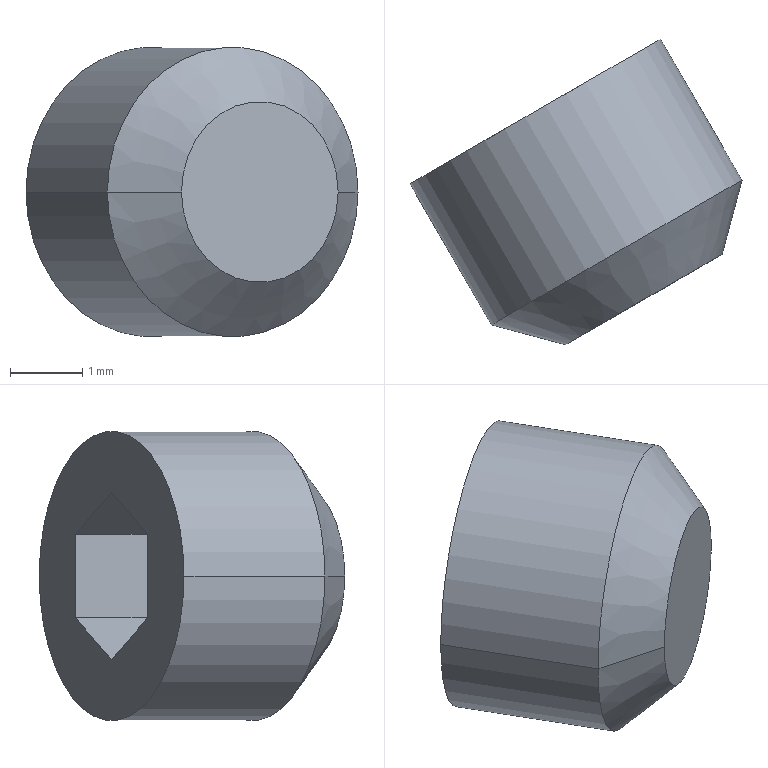Part | SolidWorks | features BaseBody 1 | 1 solid | 20 faces | box 4.589 x 4.223 x 4 mm | volume 28.806 mm3 | plane 14 | cone 4 | cylinder 2 | commonest cylinder face diameters 4 x2
STEP:
#1=CARTESIAN_POINT('',(315.686,1754.162,-1178.57));
#2=VERTEX_POINT('',#1);
#3=CARTESIAN_POINT('',(319.15,1756.162,-1178.57));
#4=VERTEX_POINT('',#3);
#5=CARTESIAN_POINT('',(317.418,1755.162,-1178.57));
#6=DIRECTION('',(-0.5,0.866,0.));
#7=DIRECTION('',(-0.866,-0.5,0.));
#8=AXIS2_PLACEMENT_3D('',#5,#6,#7);
#9=CIRCLE('',#8,2.);
#10=EDGE_CURVE('',#2,#4,#9,.T.);
#11=ORIENTED_EDGE('',*,*,#10,.T.);
#12=CARTESIAN_POINT('',(318.025,1758.11,-1178.57));
#13=VERTEX_POINT('',#12);
#14=CARTESIAN_POINT('',(318.025,1758.11,-1178.57));
#15=DIRECTION('',(-0.5,0.866,0.));
#16=VECTOR('',#15,1000.);
#17=LINE('',#14,#16);
#18=EDGE_CURVE('',#4,#13,#17,.T.);
#19=ORIENTED_EDGE('',*,*,#18,.T.);
#20=CARTESIAN_POINT('',(314.561,1756.11,-1178.57));
#21=VERTEX_POINT('',#20);
#22=CARTESIAN_POINT('',(316.293,1757.11,-1178.57));
#23=DIRECTION('',(0.5,-0.866,0.));
#24=DIRECTION('',(-0.866,-0.5,0.));
#25=AXIS2_PLACEMENT_3D('',#22,#23,#24);
#26=CIRCLE('',#25,2.);
#27=EDGE_CURVE('',#13,#21,#26,.T.);
#28=ORIENTED_EDGE('',*,*,#27,.T.);
#29=CARTESIAN_POINT('',(314.561,1756.11,-1178.57));
#30=DIRECTION('',(-0.5,0.866,0.));
#31=VECTOR('',#30,1000.);
#32=LINE('',#29,#31);
#33=EDGE_CURVE('',#2,#21,#32,.T.);
#34=ORIENTED_EDGE('',*,*,#33,.F.);
#35=EDGE_LOOP('',(#11,#19,#28,#34));
#36=FACE_OUTER_BOUND('',#35,.T.);
#37=CARTESIAN_POINT('',(316.293,1757.11,-1178.57));
#38=DIRECTION('',(-0.5,0.866,0.));
#39=DIRECTION('',(-0.866,-0.5,0.));
#40=AXIS2_PLACEMENT_3D('',#37,#38,#39);
#41=CYLINDRICAL_SURFACE('',#40,2.);
#42=ADVANCED_FACE('',(#36),#41,.T.);
#43=CARTESIAN_POINT('',(316.71,1753.887,-1178.57));
#44=VERTEX_POINT('',#43);
#45=CARTESIAN_POINT('',(318.875,1755.137,-1178.57));
#46=VERTEX_POINT('',#45);
#47=CARTESIAN_POINT('',(317.793,1754.512,-1178.57));
#48=DIRECTION('',(-0.5,0.866,0.));
#49=DIRECTION('',(-0.866,-0.5,0.));
#50=AXIS2_PLACEMENT_3D('',#47,#48,#49);
#51=CIRCLE('',#50,1.25);
#52=EDGE_CURVE('',#44,#46,#51,.T.);
#53=ORIENTED_EDGE('',*,*,#52,.T.);
#54=CARTESIAN_POINT('',(319.15,1756.162,-1178.57));
#55=DIRECTION('',(0.2588,0.9659,0.));
#56=VECTOR('',#55,1000.);
#57=LINE('',#54,#56);
#58=EDGE_CURVE('',#46,#4,#57,.T.);
#59=ORIENTED_EDGE('',*,*,#58,.T.);
#60=ORIENTED_EDGE('',*,*,#10,.F.);
#61=CARTESIAN_POINT('',(315.686,1754.162,-1178.57));
#62=DIRECTION('',(-0.9659,0.2588,0.));
#63=VECTOR('',#62,1000.);
#64=LINE('',#61,#63);
#65=EDGE_CURVE('',#44,#2,#64,.T.);
#66=ORIENTED_EDGE('',*,*,#65,.F.);
#67=EDGE_LOOP('',(#53,#59,#60,#66));
#68=FACE_OUTER_BOUND('',#67,.T.);
#69=CARTESIAN_POINT('',(317.418,1755.162,-1178.57));
#70=DIRECTION('',(-0.5,0.866,0.));
#71=DIRECTION('',(-0.866,-0.5,0.));
#72=AXIS2_PLACEMENT_3D('',#69,#70,#71);
#73=CONICAL_SURFACE('',#72,2.,0.7854);
#74=ADVANCED_FACE('',(#68),#73,.T.);
#75=CARTESIAN_POINT('',(317.331,1755.311,-1178.57));
#76=VERTEX_POINT('',#75);
#77=CARTESIAN_POINT('',(316.177,1755.311,-1178.57));
#78=VERTEX_POINT('',#77);
#79=CARTESIAN_POINT('',(316.177,1755.311,-1178.57));
#80=DIRECTION('',(-1.,0.,0.));
#81=VECTOR('',#80,1000.);
#82=LINE('',#79,#81);
#83=EDGE_CURVE('',#76,#78,#82,.T.);
#84=ORIENTED_EDGE('',*,*,#83,.F.);
#85=CARTESIAN_POINT('',(317.909,1756.311,-1178.57));
#86=VERTEX_POINT('',#85);
#87=CARTESIAN_POINT('',(317.909,1756.311,-1178.57));
#88=DIRECTION('',(0.5,0.866,0.));
#89=VECTOR('',#88,1000.);
#90=LINE('',#87,#89);
#91=EDGE_CURVE('',#76,#86,#90,.T.);
#92=ORIENTED_EDGE('',*,*,#91,.T.);
#93=CARTESIAN_POINT('',(317.476,1756.061,-1179.436));
#94=VERTEX_POINT('',#93);
#95=CARTESIAN_POINT('',(317.043,1755.811,-1178.57));
#96=DIRECTION('',(0.5,-0.866,0.));
#97=DIRECTION('',(-0.866,-0.5,0.));
#98=AXIS2_PLACEMENT_3D('',#95,#96,#97);
#99=CIRCLE('',#98,1.);
#100=EDGE_CURVE('',#94,#86,#99,.T.);
#101=ORIENTED_EDGE('',*,*,#100,.F.);
#102=CARTESIAN_POINT('',(316.61,1755.561,-1179.436));
#103=VERTEX_POINT('',#102);
#104=CARTESIAN_POINT('',(317.043,1755.811,-1178.57));
#105=DIRECTION('',(0.5,-0.866,0.));
#106=DIRECTION('',(-0.866,-0.5,0.));
#107=AXIS2_PLACEMENT_3D('',#104,#105,#106);
#108=CIRCLE('',#107,1.);
#109=EDGE_CURVE('',#103,#94,#108,.T.);
#110=ORIENTED_EDGE('',*,*,#109,.F.);
#111=CARTESIAN_POINT('',(317.043,1755.811,-1178.57));
#112=DIRECTION('',(0.5,-0.866,0.));
#113=DIRECTION('',(-0.866,-0.5,0.));
#114=AXIS2_PLACEMENT_3D('',#111,#112,#113);
#115=CIRCLE('',#114,1.);
#116=EDGE_CURVE('',#78,#103,#115,.T.);
#117=ORIENTED_EDGE('',*,*,#116,.F.);
#118=EDGE_LOOP('',(#84,#92,#101,#110,#117));
#119=FACE_OUTER_BOUND('',#118,.T.);
#120=CARTESIAN_POINT('',(317.043,1755.811,-1178.57));
#121=DIRECTION('',(-0.5,0.866,0.));
#122=DIRECTION('',(-0.866,-0.5,0.));
#123=AXIS2_PLACEMENT_3D('',#120,#121,#122);
#124=CONICAL_SURFACE('',#123,1.,1.047);
#125=ADVANCED_FACE('',(#119),#124,.F.);
#126=ORIENTED_EDGE('',*,*,#18,.F.);
#127=CARTESIAN_POINT('',(317.418,1755.162,-1178.57));
#128=DIRECTION('',(-0.5,0.866,0.));
#129=DIRECTION('',(-0.866,-0.5,0.));
#130=AXIS2_PLACEMENT_3D('',#127,#128,#129);
#131=CIRCLE('',#130,2.);
#132=EDGE_CURVE('',#4,#2,#131,.T.);
#133=ORIENTED_EDGE('',*,*,#132,.T.);
#134=ORIENTED_EDGE('',*,*,#33,.T.);
#135=CARTESIAN_POINT('',(316.293,1757.11,-1178.57));
#136=DIRECTION('',(0.5,-0.866,0.));
#137=DIRECTION('',(-0.866,-0.5,0.));
#138=AXIS2_PLACEMENT_3D('',#135,#136,#137);
#139=CIRCLE('',#138,2.);
#140=EDGE_CURVE('',#21,#13,#139,.T.);
#141=ORIENTED_EDGE('',*,*,#140,.T.);
#142=EDGE_LOOP('',(#126,#133,#134,#141));
#143=FACE_OUTER_BOUND('',#142,.T.);
#144=CARTESIAN_POINT('',(316.293,1757.11,-1178.57));
#145=DIRECTION('',(-0.5,0.866,0.));
#146=DIRECTION('',(-0.866,-0.5,0.));
#147=AXIS2_PLACEMENT_3D('',#144,#145,#146);
#148=CYLINDRICAL_SURFACE('',#147,2.);
#149=ADVANCED_FACE('',(#143),#148,.T.);
#150=CARTESIAN_POINT('',(317.159,1757.61,-1177.993));
#151=VERTEX_POINT('',#150);
#152=CARTESIAN_POINT('',(317.159,1757.61,-1179.147));
#153=VERTEX_POINT('',#152);
#154=CARTESIAN_POINT('',(317.159,1757.61,-1178.57));
#155=DIRECTION('',(0.,0.,-1.));
#156=VECTOR('',#155,1000.);
#157=LINE('',#154,#156);
#158=EDGE_CURVE('',#151,#153,#157,.T.);
#159=ORIENTED_EDGE('',*,*,#158,.F.);
#160=CARTESIAN_POINT('',(316.293,1757.11,-1177.415));
#161=VERTEX_POINT('',#160);
#162=CARTESIAN_POINT('',(316.293,1757.11,-1177.415));
#163=DIRECTION('',(0.75,0.433,-0.5));
#164=VECTOR('',#163,1000.);
#165=LINE('',#162,#164);
#166=EDGE_CURVE('',#161,#151,#165,.T.);
#167=ORIENTED_EDGE('',*,*,#166,.F.);
#168=CARTESIAN_POINT('',(315.427,1756.61,-1177.993));
#169=VERTEX_POINT('',#168);
#170=CARTESIAN_POINT('',(315.427,1756.61,-1177.993));
#171=DIRECTION('',(0.75,0.433,0.5));
#172=VECTOR('',#171,1000.);
#173=LINE('',#170,#172);
#174=EDGE_CURVE('',#169,#161,#173,.T.);
#175=ORIENTED_EDGE('',*,*,#174,.F.);
#176=CARTESIAN_POINT('',(315.427,1756.61,-1179.147));
#177=VERTEX_POINT('',#176);
#178=CARTESIAN_POINT('',(315.427,1756.61,-1178.57));
#179=DIRECTION('',(0.,0.,1.));
#180=VECTOR('',#179,1000.);
#181=LINE('',#178,#180);
#182=EDGE_CURVE('',#177,#169,#181,.T.);
#183=ORIENTED_EDGE('',*,*,#182,.F.);
#184=CARTESIAN_POINT('',(316.293,1757.11,-1179.725));
#185=VERTEX_POINT('',#184);
#186=CARTESIAN_POINT('',(316.293,1757.11,-1179.725));
#187=DIRECTION('',(-0.75,-0.433,0.5));
#188=VECTOR('',#187,1000.);
#189=LINE('',#186,#188);
#190=EDGE_CURVE('',#185,#177,#189,.T.);
#191=ORIENTED_EDGE('',*,*,#190,.F.);
#192=CARTESIAN_POINT('',(317.159,1757.61,-1179.147));
#193=DIRECTION('',(-0.75,-0.433,-0.5));
#194=VECTOR('',#193,1000.);
#195=LINE('',#192,#194);
#196=EDGE_CURVE('',#153,#185,#195,.T.);
#197=ORIENTED_EDGE('',*,*,#196,.F.);
#198=EDGE_LOOP('',(#159,#167,#175,#183,#191,#197));
#199=FACE_BOUND('',#198,.T.);
#200=ORIENTED_EDGE('',*,*,#140,.F.);
#201=ORIENTED_EDGE('',*,*,#27,.F.);
#202=EDGE_LOOP('',(#200,#201));
#203=FACE_OUTER_BOUND('',#202,.T.);
#204=CARTESIAN_POINT('',(316.293,1757.11,-1178.57));
#205=DIRECTION('',(0.5,-0.866,0.));
#206=DIRECTION('',(0.866,0.5,0.));
#207=AXIS2_PLACEMENT_3D('',#204,#205,#206);
#208=PLANE('',#207);
#209=ADVANCED_FACE('',(#199,#203),#208,.F.);
#210=ORIENTED_EDGE('',*,*,#58,.F.);
#211=CARTESIAN_POINT('',(317.793,1754.512,-1178.57));
#212=DIRECTION('',(-0.5,0.866,0.));
#213=DIRECTION('',(-0.866,-0.5,0.));
#214=AXIS2_PLACEMENT_3D('',#211,#212,#213);
#215=CIRCLE('',#214,1.25);
#216=EDGE_CURVE('',#46,#44,#215,.T.);
#217=ORIENTED_EDGE('',*,*,#216,.T.);
#218=ORIENTED_EDGE('',*,*,#65,.T.);
#219=ORIENTED_EDGE('',*,*,#132,.F.);
#220=EDGE_LOOP('',(#210,#217,#218,#219));
#221=FACE_OUTER_BOUND('',#220,.T.);
#222=CARTESIAN_POINT('',(317.418,1755.162,-1178.57));
#223=DIRECTION('',(-0.5,0.866,0.));
#224=DIRECTION('',(-0.866,-0.5,0.));
#225=AXIS2_PLACEMENT_3D('',#222,#223,#224);
#226=CONICAL_SURFACE('',#225,2.,0.7854);
#227=ADVANCED_FACE('',(#221),#226,.T.);
#228=ORIENTED_EDGE('',*,*,#196,.T.);
#229=CARTESIAN_POINT('',(317.043,1755.811,-1179.725));
#230=VERTEX_POINT('',#229);
#231=CARTESIAN_POINT('',(317.043,1755.811,-1179.725));
#232=DIRECTION('',(-0.5,0.866,0.));
#233=VECTOR('',#232,1000.);
#234=LINE('',#231,#233);
#235=EDGE_CURVE('',#230,#185,#234,.T.);
#236=ORIENTED_EDGE('',*,*,#235,.F.);
#237=CARTESIAN_POINT('',(317.476,1756.061,-1179.436));
#238=DIRECTION('',(-0.75,-0.433,-0.5));
#239=VECTOR('',#238,1000.);
#240=LINE('',#237,#239);
#241=EDGE_CURVE('',#94,#230,#240,.T.);
#242=ORIENTED_EDGE('',*,*,#241,.F.);
#243=CARTESIAN_POINT('',(317.909,1756.311,-1179.147));
#244=VERTEX_POINT('',#243);
#245=CARTESIAN_POINT('',(317.909,1756.311,-1179.147));
#246=DIRECTION('',(-0.75,-0.433,-0.5));
#247=VECTOR('',#246,1000.);
#248=LINE('',#245,#247);
#249=EDGE_CURVE('',#244,#94,#248,.T.);
#250=ORIENTED_EDGE('',*,*,#249,.F.);
#251=CARTESIAN_POINT('',(317.159,1757.61,-1179.147));
#252=DIRECTION('',(0.5,-0.866,0.));
#253=VECTOR('',#252,1000.);
#254=LINE('',#251,#253);
#255=EDGE_CURVE('',#153,#244,#254,.T.);
#256=ORIENTED_EDGE('',*,*,#255,.F.);
#257=EDGE_LOOP('',(#228,#236,#242,#250,#256));
#258=FACE_OUTER_BOUND('',#257,.T.);
#259=CARTESIAN_POINT('',(317.909,1756.311,-1179.147));
#260=DIRECTION('',(0.433,0.25,-0.866));
#261=DIRECTION('',(-0.8944,0.,-0.4472));
#262=AXIS2_PLACEMENT_3D('',#259,#260,#261);
#263=PLANE('',#262);
#264=ADVANCED_FACE('',(#258),#263,.F.);
#265=ORIENTED_EDGE('',*,*,#158,.T.);
#266=ORIENTED_EDGE('',*,*,#255,.T.);
#267=CARTESIAN_POINT('',(317.909,1756.311,-1177.993));
#268=DIRECTION('',(0.,0.,-1.));
#269=VECTOR('',#268,1000.);
#270=LINE('',#267,#269);
#271=EDGE_CURVE('',#86,#244,#270,.T.);
#272=ORIENTED_EDGE('',*,*,#271,.F.);
#273=CARTESIAN_POINT('',(317.909,1756.311,-1177.993));
#274=VERTEX_POINT('',#273);
#275=CARTESIAN_POINT('',(317.909,1756.311,-1177.993));
#276=DIRECTION('',(0.,0.,-1.));
#277=VECTOR('',#276,1000.);
#278=LINE('',#275,#277);
#279=EDGE_CURVE('',#274,#86,#278,.T.);
#280=ORIENTED_EDGE('',*,*,#279,.F.);
#281=CARTESIAN_POINT('',(317.909,1756.311,-1177.993));
#282=DIRECTION('',(0.5,-0.866,0.));
#283=VECTOR('',#282,1000.);
#284=LINE('',#281,#283);
#285=EDGE_CURVE('',#151,#274,#284,.T.);
#286=ORIENTED_EDGE('',*,*,#285,.F.);
#287=EDGE_LOOP('',(#265,#266,#272,#280,#286));
#288=FACE_OUTER_BOUND('',#287,.T.);
#289=CARTESIAN_POINT('',(317.909,1756.311,-1177.993));
#290=DIRECTION('',(0.866,0.5,0.));
#291=DIRECTION('',(-0.5,0.866,0.));
#292=AXIS2_PLACEMENT_3D('',#289,#290,#291);
#293=PLANE('',#292);
#294=ADVANCED_FACE('',(#288),#293,.F.);
#295=ORIENTED_EDGE('',*,*,#166,.T.);
#296=ORIENTED_EDGE('',*,*,#285,.T.);
#297=CARTESIAN_POINT('',(317.476,1756.061,-1177.704));
#298=VERTEX_POINT('',#297);
#299=CARTESIAN_POINT('',(317.476,1756.061,-1177.704));
#300=DIRECTION('',(0.75,0.433,-0.5));
#301=VECTOR('',#300,1000.);
#302=LINE('',#299,#301);
#303=EDGE_CURVE('',#298,#274,#302,.T.);
#304=ORIENTED_EDGE('',*,*,#303,.F.);
#305=CARTESIAN_POINT('',(317.043,1755.811,-1177.415));
#306=VERTEX_POINT('',#305);
#307=CARTESIAN_POINT('',(317.043,1755.811,-1177.415));
#308=DIRECTION('',(0.75,0.433,-0.5));
#309=VECTOR('',#308,1000.);
#310=LINE('',#307,#309);
#311=EDGE_CURVE('',#306,#298,#310,.T.);
#312=ORIENTED_EDGE('',*,*,#311,.F.);
#313=CARTESIAN_POINT('',(316.293,1757.11,-1177.415));
#314=DIRECTION('',(0.5,-0.866,0.));
#315=VECTOR('',#314,1000.);
#316=LINE('',#313,#315);
#317=EDGE_CURVE('',#161,#306,#316,.T.);
#318=ORIENTED_EDGE('',*,*,#317,.F.);
#319=EDGE_LOOP('',(#295,#296,#304,#312,#318));
#320=FACE_OUTER_BOUND('',#319,.T.);
#321=CARTESIAN_POINT('',(317.043,1755.811,-1177.415));
#322=DIRECTION('',(0.433,0.25,0.866));
#323=DIRECTION('',(0.8944,0.,-0.4472));
#324=AXIS2_PLACEMENT_3D('',#321,#322,#323);
#325=PLANE('',#324);
#326=ADVANCED_FACE('',(#320),#325,.F.);
#327=ORIENTED_EDGE('',*,*,#174,.T.);
#328=ORIENTED_EDGE('',*,*,#317,.T.);
#329=CARTESIAN_POINT('',(316.61,1755.561,-1177.704));
#330=VERTEX_POINT('',#329);
#331=CARTESIAN_POINT('',(316.61,1755.561,-1177.704));
#332=DIRECTION('',(0.75,0.433,0.5));
#333=VECTOR('',#332,1000.);
#334=LINE('',#331,#333);
#335=EDGE_CURVE('',#330,#306,#334,.T.);
#336=ORIENTED_EDGE('',*,*,#335,.F.);
#337=CARTESIAN_POINT('',(316.177,1755.311,-1177.993));
#338=VERTEX_POINT('',#337);
#339=CARTESIAN_POINT('',(316.177,1755.311,-1177.993));
#340=DIRECTION('',(0.75,0.433,0.5));
#341=VECTOR('',#340,1000.);
#342=LINE('',#339,#341);
#343=EDGE_CURVE('',#338,#330,#342,.T.);
#344=ORIENTED_EDGE('',*,*,#343,.F.);
#345=CARTESIAN_POINT('',(315.427,1756.61,-1177.993));
#346=DIRECTION('',(0.5,-0.866,0.));
#347=VECTOR('',#346,1000.);
#348=LINE('',#345,#347);
#349=EDGE_CURVE('',#169,#338,#348,.T.);
#350=ORIENTED_EDGE('',*,*,#349,.F.);
#351=EDGE_LOOP('',(#327,#328,#336,#344,#350));
#352=FACE_OUTER_BOUND('',#351,.T.);
#353=CARTESIAN_POINT('',(316.177,1755.311,-1177.993));
#354=DIRECTION('',(-0.433,-0.25,0.866));
#355=DIRECTION('',(0.8944,0.,0.4472));
#356=AXIS2_PLACEMENT_3D('',#353,#354,#355);
#357=PLANE('',#356);
#358=ADVANCED_FACE('',(#352),#357,.F.);
#359=ORIENTED_EDGE('',*,*,#182,.T.);
#360=ORIENTED_EDGE('',*,*,#349,.T.);
#361=CARTESIAN_POINT('',(316.177,1755.311,-1179.147));
#362=DIRECTION('',(0.,0.,1.));
#363=VECTOR('',#362,1000.);
#364=LINE('',#361,#363);
#365=EDGE_CURVE('',#78,#338,#364,.T.);
#366=ORIENTED_EDGE('',*,*,#365,.F.);
#367=CARTESIAN_POINT('',(316.177,1755.311,-1179.147));
#368=VERTEX_POINT('',#367);
#369=CARTESIAN_POINT('',(316.177,1755.311,-1179.147));
#370=DIRECTION('',(0.,0.,1.));
#371=VECTOR('',#370,1000.);
#372=LINE('',#369,#371);
#373=EDGE_CURVE('',#368,#78,#372,.T.);
#374=ORIENTED_EDGE('',*,*,#373,.F.);
#375=CARTESIAN_POINT('',(316.177,1755.311,-1179.147));
#376=DIRECTION('',(0.5,-0.866,0.));
#377=VECTOR('',#376,1000.);
#378=LINE('',#375,#377);
#379=EDGE_CURVE('',#177,#368,#378,.T.);
#380=ORIENTED_EDGE('',*,*,#379,.F.);
#381=EDGE_LOOP('',(#359,#360,#366,#374,#380));
#382=FACE_OUTER_BOUND('',#381,.T.);
#383=CARTESIAN_POINT('',(316.177,1755.311,-1179.147));
#384=DIRECTION('',(-0.866,-0.5,0.));
#385=DIRECTION('',(0.5,-0.866,0.));
#386=AXIS2_PLACEMENT_3D('',#383,#384,#385);
#387=PLANE('',#386);
#388=ADVANCED_FACE('',(#382),#387,.F.);
#389=ORIENTED_EDGE('',*,*,#190,.T.);
#390=ORIENTED_EDGE('',*,*,#379,.T.);
#391=CARTESIAN_POINT('',(316.61,1755.561,-1179.436));
#392=DIRECTION('',(-0.75,-0.433,0.5));
#393=VECTOR('',#392,1000.);
#394=LINE('',#391,#393);
#395=EDGE_CURVE('',#103,#368,#394,.T.);
#396=ORIENTED_EDGE('',*,*,#395,.F.);
#397=CARTESIAN_POINT('',(317.043,1755.811,-1179.725));
#398=DIRECTION('',(-0.75,-0.433,0.5));
#399=VECTOR('',#398,1000.);
#400=LINE('',#397,#399);
#401=EDGE_CURVE('',#230,#103,#400,.T.);
#402=ORIENTED_EDGE('',*,*,#401,.F.);
#403=ORIENTED_EDGE('',*,*,#235,.T.);
#404=EDGE_LOOP('',(#389,#390,#396,#402,#403));
#405=FACE_OUTER_BOUND('',#404,.T.);
#406=CARTESIAN_POINT('',(317.043,1755.811,-1179.725));
#407=DIRECTION('',(-0.433,-0.25,-0.866));
#408=DIRECTION('',(-0.8944,0.,0.4472));
#409=AXIS2_PLACEMENT_3D('',#406,#407,#408);
#410=PLANE('',#409);
#411=ADVANCED_FACE('',(#405),#410,.F.);
#412=ORIENTED_EDGE('',*,*,#52,.F.);
#413=ORIENTED_EDGE('',*,*,#216,.F.);
#414=EDGE_LOOP('',(#412,#413));
#415=FACE_OUTER_BOUND('',#414,.T.);
#416=CARTESIAN_POINT('',(317.793,1754.512,-1178.57));
#417=DIRECTION('',(-0.5,0.866,0.));
#418=DIRECTION('',(-0.866,-0.5,0.));
#419=AXIS2_PLACEMENT_3D('',#416,#417,#418);
#420=PLANE('',#419);
#421=ADVANCED_FACE('',(#415),#420,.F.);
#422=ORIENTED_EDGE('',*,*,#109,.T.);
#423=ORIENTED_EDGE('',*,*,#241,.T.);
#424=ORIENTED_EDGE('',*,*,#401,.T.);
#425=EDGE_LOOP('',(#422,#423,#424));
#426=FACE_OUTER_BOUND('',#425,.T.);
#427=CARTESIAN_POINT('',(317.043,1755.811,-1178.57));
#428=DIRECTION('',(-0.5,0.866,0.));
#429=DIRECTION('',(-0.866,-0.5,0.));
#430=AXIS2_PLACEMENT_3D('',#427,#428,#429);
#431=PLANE('',#430);
#432=ADVANCED_FACE('',(#426),#431,.T.);
#433=ORIENTED_EDGE('',*,*,#100,.T.);
#434=ORIENTED_EDGE('',*,*,#271,.T.);
#435=ORIENTED_EDGE('',*,*,#249,.T.);
#436=EDGE_LOOP('',(#433,#434,#435));
#437=FACE_OUTER_BOUND('',#436,.T.);
#438=CARTESIAN_POINT('',(317.043,1755.811,-1178.57));
#439=DIRECTION('',(-0.5,0.866,0.));
#440=DIRECTION('',(-0.866,-0.5,0.));
#441=AXIS2_PLACEMENT_3D('',#438,#439,#440);
#442=PLANE('',#441);
#443=ADVANCED_FACE('',(#437),#442,.T.);
#444=CARTESIAN_POINT('',(317.043,1755.811,-1178.57));
#445=DIRECTION('',(0.5,-0.866,0.));
#446=DIRECTION('',(-0.866,-0.5,0.));
#447=AXIS2_PLACEMENT_3D('',#444,#445,#446);
#448=CIRCLE('',#447,1.);
#449=EDGE_CURVE('',#86,#298,#448,.T.);
#450=ORIENTED_EDGE('',*,*,#449,.T.);
#451=ORIENTED_EDGE('',*,*,#303,.T.);
#452=ORIENTED_EDGE('',*,*,#279,.T.);
#453=EDGE_LOOP('',(#450,#451,#452));
#454=FACE_OUTER_BOUND('',#453,.T.);
#455=CARTESIAN_POINT('',(317.043,1755.811,-1178.57));
#456=DIRECTION('',(-0.5,0.866,0.));
#457=DIRECTION('',(-0.866,-0.5,0.));
#458=AXIS2_PLACEMENT_3D('',#455,#456,#457);
#459=PLANE('',#458);
#460=ADVANCED_FACE('',(#454),#459,.T.);
#461=CARTESIAN_POINT('',(317.043,1755.811,-1178.57));
#462=DIRECTION('',(0.5,-0.866,0.));
#463=DIRECTION('',(-0.866,-0.5,0.));
#464=AXIS2_PLACEMENT_3D('',#461,#462,#463);
#465=CIRCLE('',#464,1.);
#466=EDGE_CURVE('',#298,#330,#465,.T.);
#467=ORIENTED_EDGE('',*,*,#466,.T.);
#468=ORIENTED_EDGE('',*,*,#335,.T.);
#469=ORIENTED_EDGE('',*,*,#311,.T.);
#470=EDGE_LOOP('',(#467,#468,#469));
#471=FACE_OUTER_BOUND('',#470,.T.);
#472=CARTESIAN_POINT('',(317.043,1755.811,-1178.57));
#473=DIRECTION('',(-0.5,0.866,0.));
#474=DIRECTION('',(-0.866,-0.5,0.));
#475=AXIS2_PLACEMENT_3D('',#472,#473,#474);
#476=PLANE('',#475);
#477=ADVANCED_FACE('',(#471),#476,.T.);
#478=CARTESIAN_POINT('',(317.043,1755.811,-1178.57));
#479=DIRECTION('',(0.5,-0.866,0.));
#480=DIRECTION('',(-0.866,-0.5,0.));
#481=AXIS2_PLACEMENT_3D('',#478,#479,#480);
#482=CIRCLE('',#481,1.);
#483=EDGE_CURVE('',#330,#78,#482,.T.);
#484=ORIENTED_EDGE('',*,*,#483,.T.);
#485=ORIENTED_EDGE('',*,*,#365,.T.);
#486=ORIENTED_EDGE('',*,*,#343,.T.);
#487=EDGE_LOOP('',(#484,#485,#486));
#488=FACE_OUTER_BOUND('',#487,.T.);
#489=CARTESIAN_POINT('',(317.043,1755.811,-1178.57));
#490=DIRECTION('',(-0.5,0.866,0.));
#491=DIRECTION('',(-0.866,-0.5,0.));
#492=AXIS2_PLACEMENT_3D('',#489,#490,#491);
#493=PLANE('',#492);
#494=ADVANCED_FACE('',(#488),#493,.T.);
#495=ORIENTED_EDGE('',*,*,#116,.T.);
#496=ORIENTED_EDGE('',*,*,#395,.T.);
#497=ORIENTED_EDGE('',*,*,#373,.T.);
#498=EDGE_LOOP('',(#495,#496,#497));
#499=FACE_OUTER_BOUND('',#498,.T.);
#500=CARTESIAN_POINT('',(317.043,1755.811,-1178.57));
#501=DIRECTION('',(-0.5,0.866,0.));
#502=DIRECTION('',(-0.866,-0.5,0.));
#503=AXIS2_PLACEMENT_3D('',#500,#501,#502);
#504=PLANE('',#503);
#505=ADVANCED_FACE('',(#499),#504,.T.);
#506=ORIENTED_EDGE('',*,*,#91,.F.);
#507=ORIENTED_EDGE('',*,*,#83,.T.);
#508=ORIENTED_EDGE('',*,*,#483,.F.);
#509=ORIENTED_EDGE('',*,*,#466,.F.);
#510=ORIENTED_EDGE('',*,*,#449,.F.);
#511=EDGE_LOOP('',(#506,#507,#508,#509,#510));
#512=FACE_OUTER_BOUND('',#511,.T.);
#513=CARTESIAN_POINT('',(317.043,1755.811,-1178.57));
#514=DIRECTION('',(-0.5,0.866,0.));
#515=DIRECTION('',(-0.866,-0.5,0.));
#516=AXIS2_PLACEMENT_3D('',#513,#514,#515);
#517=CONICAL_SURFACE('',#516,1.,1.047);
#518=ADVANCED_FACE('',(#512),#517,.F.);
#519=CLOSED_SHELL('',(#42,#74,#125,#149,#209,#227,#264,#294,#326,#358,#388,#411,#421,#432,#443,#460,#477,#494,#505,#518));
#520=MANIFOLD_SOLID_BREP('',#519);
#521=CARTESIAN_POINT('',(0.,0.,0.));
#522=DIRECTION('',(0.,0.,1.));
#523=DIRECTION('',(1.,0.,0.));
#524=AXIS2_PLACEMENT_3D('',#521,#522,#523);
#525=(LENGTH_UNIT()NAMED_UNIT(*)SI_UNIT(.MILLI.,.METRE.));
#526=UNCERTAINTY_MEASURE_WITH_UNIT(LENGTH_MEASURE(0.00001),#525,'','');
#527=(NAMED_UNIT(*)PLANE_ANGLE_UNIT()SI_UNIT($,.RADIAN.));
#528=(NAMED_UNIT(*)SI_UNIT($,.STERADIAN.)SOLID_ANGLE_UNIT());
#529=(GEOMETRIC_REPRESENTATION_CONTEXT(3)GLOBAL_UNCERTAINTY_ASSIGNED_CONTEXT((#526))GLOBAL_UNIT_ASSIGNED_CONTEXT((#525,#527,#528))REPRESENTATION_CONTEXT('',''));
#530=ADVANCED_BREP_SHAPE_REPRESENTATION('',(#520,#524),#529);